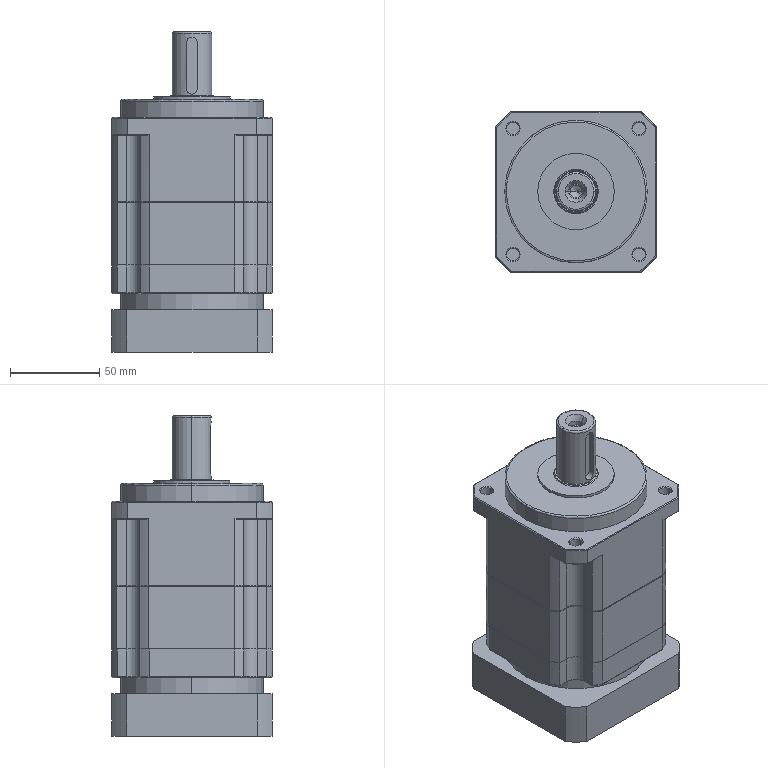Part | SolidWorks | features BaseBody 7 | 7 solids | 505 faces | box 90 x 90.211 x 179.85 mm | volume 785388 mm3 | cylinder 188 | plane 155 | cone 144 | spline 18 | commonest cylinder face diameters 102 x24 4.2 x20 5.5 x20 9 x12 15 x12 4 x8